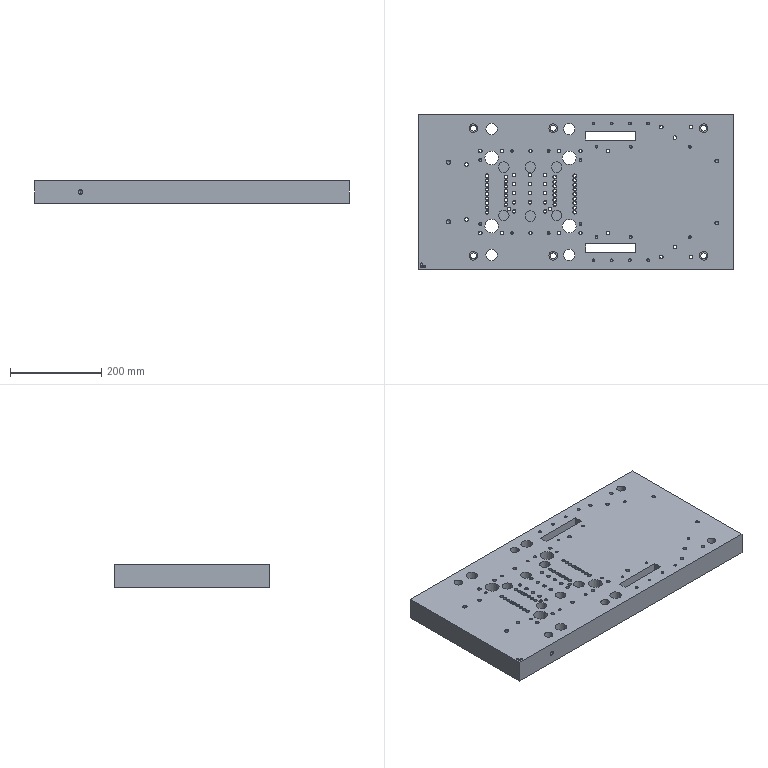Part | STEP file | 200 mesh_id2082 | 1 solid | 323 faces | box 690 x 340 x 50 mm | volume 10962643 mm3 | cone 175 | cylinder 122 | plane 26 | commonest cylinder face diameters 6.8 x60 5 x22 8.01 x10 13 x6 19 x6 23 x6